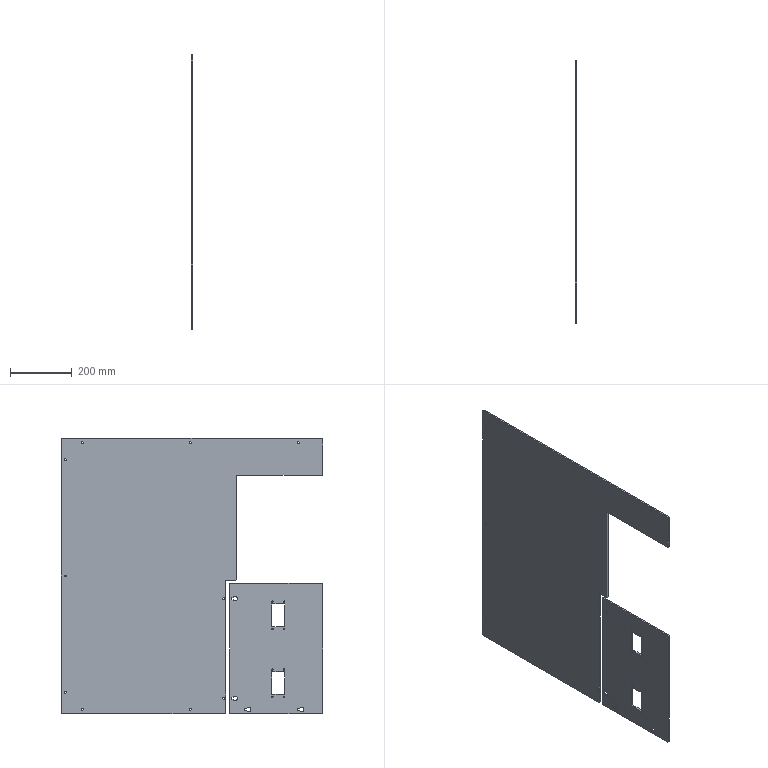Part | STEP file | 227H056116 Side Cover _Default | 2 solids | 102 faces | box 5 x 849 x 893 mm | volume 3234817 mm3 | cylinder 56 | plane 42 | cone 4 | commonest cylinder face diameters 6 x24 4.5 x16 14 x12 3.5 x4